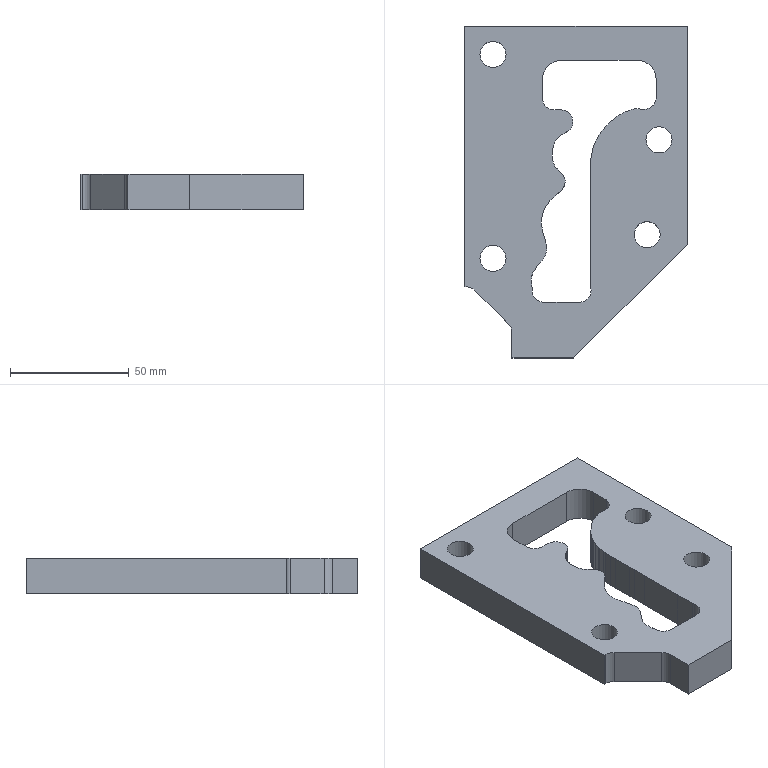Part | STEP file | 1 solid | 193 faces | box 94 x 140 x 15 mm | volume 130830 mm3 | plane 178 | cylinder 15 | commonest cylinder face diameters 10 x6 11 x4 8 x3 16 x2